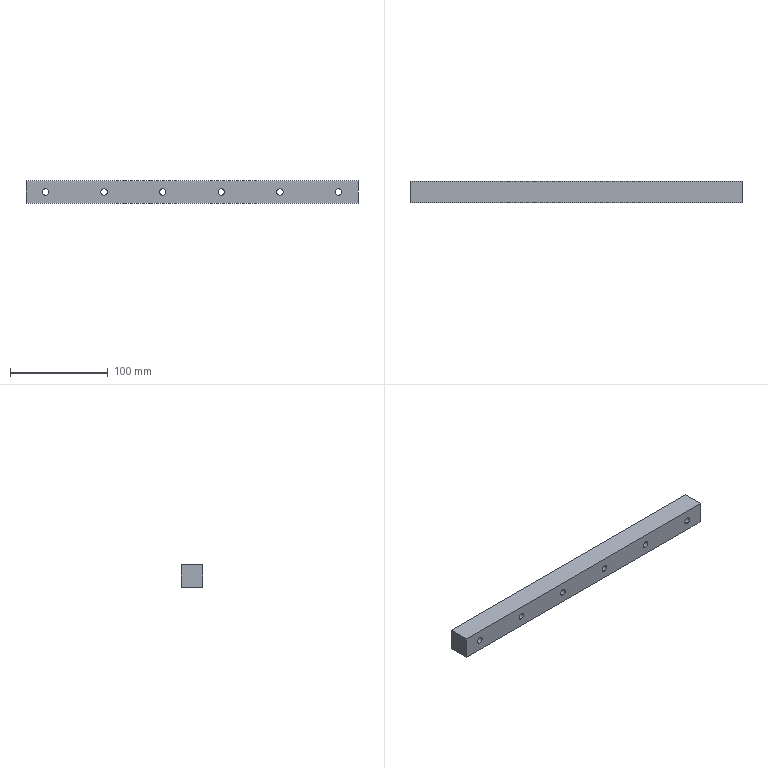Part | SolidWorks | features Extrusion 1, HoleWzd 1, LPattern 1 | 1 solid | 36 faces | box 340 x 22 x 23 mm | volume 165043 mm3 | cylinder 24 | plane 12 | commonest cylinder face diameters 6.6 x12 11 x12
STEP:
#1=CARTESIAN_POINT('',(80.,4.2,-5.5));
#2=VERTEX_POINT('',#1);
#3=CARTESIAN_POINT('',(80.,4.2,5.5));
#4=VERTEX_POINT('',#3);
#5=CARTESIAN_POINT('',(80.,4.2,0.));
#6=DIRECTION('',(0.,1.,0.));
#7=DIRECTION('',(0.,0.,1.));
#8=AXIS2_PLACEMENT_3D('',#5,#6,#7);
#9=CIRCLE('',#8,5.5);
#10=EDGE_CURVE('',#2,#4,#9,.T.);
#11=ORIENTED_EDGE('',*,*,#10,.F.);
#12=CARTESIAN_POINT('',(80.,11.,-5.5));
#13=VERTEX_POINT('',#12);
#14=CARTESIAN_POINT('',(80.,11.,-5.5));
#15=DIRECTION('',(0.,1.,0.));
#16=VECTOR('',#15,1000.);
#17=LINE('',#14,#16);
#18=EDGE_CURVE('',#2,#13,#17,.T.);
#19=ORIENTED_EDGE('',*,*,#18,.T.);
#20=CARTESIAN_POINT('',(80.,11.,5.5));
#21=VERTEX_POINT('',#20);
#22=CARTESIAN_POINT('',(80.,11.,0.));
#23=DIRECTION('',(0.,1.,0.));
#24=DIRECTION('',(0.,0.,1.));
#25=AXIS2_PLACEMENT_3D('',#22,#23,#24);
#26=CIRCLE('',#25,5.5);
#27=EDGE_CURVE('',#13,#21,#26,.T.);
#28=ORIENTED_EDGE('',*,*,#27,.T.);
#29=CARTESIAN_POINT('',(80.,11.,5.5));
#30=DIRECTION('',(0.,1.,0.));
#31=VECTOR('',#30,1000.);
#32=LINE('',#29,#31);
#33=EDGE_CURVE('',#4,#21,#32,.T.);
#34=ORIENTED_EDGE('',*,*,#33,.F.);
#35=EDGE_LOOP('',(#11,#19,#28,#34));
#36=FACE_OUTER_BOUND('',#35,.T.);
#37=CARTESIAN_POINT('',(80.,11.,0.));
#38=DIRECTION('',(0.,1.,0.));
#39=DIRECTION('',(0.,0.,1.));
#40=AXIS2_PLACEMENT_3D('',#37,#38,#39);
#41=CYLINDRICAL_SURFACE('',#40,5.5);
#42=ADVANCED_FACE('',(#36),#41,.F.);
#43=CARTESIAN_POINT('',(80.,-11.,-3.3));
#44=VERTEX_POINT('',#43);
#45=CARTESIAN_POINT('',(80.,-11.,3.3));
#46=VERTEX_POINT('',#45);
#47=CARTESIAN_POINT('',(80.,-11.,0.));
#48=DIRECTION('',(0.,1.,0.));
#49=DIRECTION('',(0.,0.,1.));
#50=AXIS2_PLACEMENT_3D('',#47,#48,#49);
#51=CIRCLE('',#50,3.3);
#52=EDGE_CURVE('',#44,#46,#51,.T.);
#53=ORIENTED_EDGE('',*,*,#52,.F.);
#54=CARTESIAN_POINT('',(80.,4.2,-3.3));
#55=VERTEX_POINT('',#54);
#56=CARTESIAN_POINT('',(80.,11.,-3.3));
#57=DIRECTION('',(0.,1.,0.));
#58=VECTOR('',#57,1000.);
#59=LINE('',#56,#58);
#60=EDGE_CURVE('',#44,#55,#59,.T.);
#61=ORIENTED_EDGE('',*,*,#60,.T.);
#62=CARTESIAN_POINT('',(80.,4.2,3.3));
#63=VERTEX_POINT('',#62);
#64=CARTESIAN_POINT('',(80.,4.2,0.));
#65=DIRECTION('',(0.,1.,0.));
#66=DIRECTION('',(0.,0.,1.));
#67=AXIS2_PLACEMENT_3D('',#64,#65,#66);
#68=CIRCLE('',#67,3.3);
#69=EDGE_CURVE('',#55,#63,#68,.T.);
#70=ORIENTED_EDGE('',*,*,#69,.T.);
#71=CARTESIAN_POINT('',(80.,11.,3.3));
#72=DIRECTION('',(0.,1.,0.));
#73=VECTOR('',#72,1000.);
#74=LINE('',#71,#73);
#75=EDGE_CURVE('',#46,#63,#74,.T.);
#76=ORIENTED_EDGE('',*,*,#75,.F.);
#77=EDGE_LOOP('',(#53,#61,#70,#76));
#78=FACE_OUTER_BOUND('',#77,.T.);
#79=CARTESIAN_POINT('',(80.,11.,0.));
#80=DIRECTION('',(0.,1.,0.));
#81=DIRECTION('',(0.,0.,1.));
#82=AXIS2_PLACEMENT_3D('',#79,#80,#81);
#83=CYLINDRICAL_SURFACE('',#82,3.3);
#84=ADVANCED_FACE('',(#78),#83,.F.);
#85=CARTESIAN_POINT('',(20.,4.2,-5.5));
#86=VERTEX_POINT('',#85);
#87=CARTESIAN_POINT('',(20.,4.2,5.5));
#88=VERTEX_POINT('',#87);
#89=CARTESIAN_POINT('',(20.,4.2,0.));
#90=DIRECTION('',(0.,1.,0.));
#91=DIRECTION('',(0.,0.,1.));
#92=AXIS2_PLACEMENT_3D('',#89,#90,#91);
#93=CIRCLE('',#92,5.5);
#94=EDGE_CURVE('',#86,#88,#93,.T.);
#95=ORIENTED_EDGE('',*,*,#94,.F.);
#96=CARTESIAN_POINT('',(20.,11.,-5.5));
#97=VERTEX_POINT('',#96);
#98=CARTESIAN_POINT('',(20.,11.,-5.5));
#99=DIRECTION('',(0.,1.,0.));
#100=VECTOR('',#99,1000.);
#101=LINE('',#98,#100);
#102=EDGE_CURVE('',#86,#97,#101,.T.);
#103=ORIENTED_EDGE('',*,*,#102,.T.);
#104=CARTESIAN_POINT('',(20.,11.,5.5));
#105=VERTEX_POINT('',#104);
#106=CARTESIAN_POINT('',(20.,11.,0.));
#107=DIRECTION('',(0.,1.,0.));
#108=DIRECTION('',(0.,0.,1.));
#109=AXIS2_PLACEMENT_3D('',#106,#107,#108);
#110=CIRCLE('',#109,5.5);
#111=EDGE_CURVE('',#97,#105,#110,.T.);
#112=ORIENTED_EDGE('',*,*,#111,.T.);
#113=CARTESIAN_POINT('',(20.,11.,5.5));
#114=DIRECTION('',(0.,1.,0.));
#115=VECTOR('',#114,1000.);
#116=LINE('',#113,#115);
#117=EDGE_CURVE('',#88,#105,#116,.T.);
#118=ORIENTED_EDGE('',*,*,#117,.F.);
#119=EDGE_LOOP('',(#95,#103,#112,#118));
#120=FACE_OUTER_BOUND('',#119,.T.);
#121=CARTESIAN_POINT('',(20.,11.,0.));
#122=DIRECTION('',(0.,1.,0.));
#123=DIRECTION('',(0.,0.,1.));
#124=AXIS2_PLACEMENT_3D('',#121,#122,#123);
#125=CYLINDRICAL_SURFACE('',#124,5.5);
#126=ADVANCED_FACE('',(#120),#125,.F.);
#127=CARTESIAN_POINT('',(20.,-11.,-3.3));
#128=VERTEX_POINT('',#127);
#129=CARTESIAN_POINT('',(20.,-11.,3.3));
#130=VERTEX_POINT('',#129);
#131=CARTESIAN_POINT('',(20.,-11.,0.));
#132=DIRECTION('',(0.,1.,0.));
#133=DIRECTION('',(0.,0.,1.));
#134=AXIS2_PLACEMENT_3D('',#131,#132,#133);
#135=CIRCLE('',#134,3.3);
#136=EDGE_CURVE('',#128,#130,#135,.T.);
#137=ORIENTED_EDGE('',*,*,#136,.F.);
#138=CARTESIAN_POINT('',(20.,4.2,-3.3));
#139=VERTEX_POINT('',#138);
#140=CARTESIAN_POINT('',(20.,11.,-3.3));
#141=DIRECTION('',(0.,1.,0.));
#142=VECTOR('',#141,1000.);
#143=LINE('',#140,#142);
#144=EDGE_CURVE('',#128,#139,#143,.T.);
#145=ORIENTED_EDGE('',*,*,#144,.T.);
#146=CARTESIAN_POINT('',(20.,4.2,3.3));
#147=VERTEX_POINT('',#146);
#148=CARTESIAN_POINT('',(20.,4.2,0.));
#149=DIRECTION('',(0.,1.,0.));
#150=DIRECTION('',(0.,0.,1.));
#151=AXIS2_PLACEMENT_3D('',#148,#149,#150);
#152=CIRCLE('',#151,3.3);
#153=EDGE_CURVE('',#139,#147,#152,.T.);
#154=ORIENTED_EDGE('',*,*,#153,.T.);
#155=CARTESIAN_POINT('',(20.,11.,3.3));
#156=DIRECTION('',(0.,1.,0.));
#157=VECTOR('',#156,1000.);
#158=LINE('',#155,#157);
#159=EDGE_CURVE('',#130,#147,#158,.T.);
#160=ORIENTED_EDGE('',*,*,#159,.F.);
#161=EDGE_LOOP('',(#137,#145,#154,#160));
#162=FACE_OUTER_BOUND('',#161,.T.);
#163=CARTESIAN_POINT('',(20.,11.,0.));
#164=DIRECTION('',(0.,1.,0.));
#165=DIRECTION('',(0.,0.,1.));
#166=AXIS2_PLACEMENT_3D('',#163,#164,#165);
#167=CYLINDRICAL_SURFACE('',#166,3.3);
#168=ADVANCED_FACE('',(#162),#167,.F.);
#169=CARTESIAN_POINT('',(140.,-11.,-3.3));
#170=VERTEX_POINT('',#169);
#171=CARTESIAN_POINT('',(140.,-11.,3.3));
#172=VERTEX_POINT('',#171);
#173=CARTESIAN_POINT('',(140.,-11.,0.));
#174=DIRECTION('',(0.,1.,0.));
#175=DIRECTION('',(0.,0.,1.));
#176=AXIS2_PLACEMENT_3D('',#173,#174,#175);
#177=CIRCLE('',#176,3.3);
#178=EDGE_CURVE('',#170,#172,#177,.T.);
#179=ORIENTED_EDGE('',*,*,#178,.F.);
#180=CARTESIAN_POINT('',(140.,4.2,-3.3));
#181=VERTEX_POINT('',#180);
#182=CARTESIAN_POINT('',(140.,11.,-3.3));
#183=DIRECTION('',(0.,1.,0.));
#184=VECTOR('',#183,1000.);
#185=LINE('',#182,#184);
#186=EDGE_CURVE('',#170,#181,#185,.T.);
#187=ORIENTED_EDGE('',*,*,#186,.T.);
#188=CARTESIAN_POINT('',(140.,4.2,3.3));
#189=VERTEX_POINT('',#188);
#190=CARTESIAN_POINT('',(140.,4.2,0.));
#191=DIRECTION('',(0.,1.,0.));
#192=DIRECTION('',(0.,0.,1.));
#193=AXIS2_PLACEMENT_3D('',#190,#191,#192);
#194=CIRCLE('',#193,3.3);
#195=EDGE_CURVE('',#181,#189,#194,.T.);
#196=ORIENTED_EDGE('',*,*,#195,.T.);
#197=CARTESIAN_POINT('',(140.,11.,3.3));
#198=DIRECTION('',(0.,1.,0.));
#199=VECTOR('',#198,1000.);
#200=LINE('',#197,#199);
#201=EDGE_CURVE('',#172,#189,#200,.T.);
#202=ORIENTED_EDGE('',*,*,#201,.F.);
#203=EDGE_LOOP('',(#179,#187,#196,#202));
#204=FACE_OUTER_BOUND('',#203,.T.);
#205=CARTESIAN_POINT('',(140.,11.,0.));
#206=DIRECTION('',(0.,1.,0.));
#207=DIRECTION('',(0.,0.,1.));
#208=AXIS2_PLACEMENT_3D('',#205,#206,#207);
#209=CYLINDRICAL_SURFACE('',#208,3.3);
#210=ADVANCED_FACE('',(#204),#209,.F.);
#211=CARTESIAN_POINT('',(140.,4.2,-5.5));
#212=VERTEX_POINT('',#211);
#213=CARTESIAN_POINT('',(140.,4.2,5.5));
#214=VERTEX_POINT('',#213);
#215=CARTESIAN_POINT('',(140.,4.2,0.));
#216=DIRECTION('',(0.,1.,0.));
#217=DIRECTION('',(0.,0.,1.));
#218=AXIS2_PLACEMENT_3D('',#215,#216,#217);
#219=CIRCLE('',#218,5.5);
#220=EDGE_CURVE('',#212,#214,#219,.T.);
#221=ORIENTED_EDGE('',*,*,#220,.F.);
#222=CARTESIAN_POINT('',(140.,11.,-5.5));
#223=VERTEX_POINT('',#222);
#224=CARTESIAN_POINT('',(140.,11.,-5.5));
#225=DIRECTION('',(0.,1.,0.));
#226=VECTOR('',#225,1000.);
#227=LINE('',#224,#226);
#228=EDGE_CURVE('',#212,#223,#227,.T.);
#229=ORIENTED_EDGE('',*,*,#228,.T.);
#230=CARTESIAN_POINT('',(140.,11.,5.5));
#231=VERTEX_POINT('',#230);
#232=CARTESIAN_POINT('',(140.,11.,0.));
#233=DIRECTION('',(0.,1.,0.));
#234=DIRECTION('',(0.,0.,1.));
#235=AXIS2_PLACEMENT_3D('',#232,#233,#234);
#236=CIRCLE('',#235,5.5);
#237=EDGE_CURVE('',#223,#231,#236,.T.);
#238=ORIENTED_EDGE('',*,*,#237,.T.);
#239=CARTESIAN_POINT('',(140.,11.,5.5));
#240=DIRECTION('',(0.,1.,0.));
#241=VECTOR('',#240,1000.);
#242=LINE('',#239,#241);
#243=EDGE_CURVE('',#214,#231,#242,.T.);
#244=ORIENTED_EDGE('',*,*,#243,.F.);
#245=EDGE_LOOP('',(#221,#229,#238,#244));
#246=FACE_OUTER_BOUND('',#245,.T.);
#247=CARTESIAN_POINT('',(140.,11.,0.));
#248=DIRECTION('',(0.,1.,0.));
#249=DIRECTION('',(0.,0.,1.));
#250=AXIS2_PLACEMENT_3D('',#247,#248,#249);
#251=CYLINDRICAL_SURFACE('',#250,5.5);
#252=ADVANCED_FACE('',(#246),#251,.F.);
#253=CARTESIAN_POINT('',(200.,-11.,-3.3));
#254=VERTEX_POINT('',#253);
#255=CARTESIAN_POINT('',(200.,-11.,3.3));
#256=VERTEX_POINT('',#255);
#257=CARTESIAN_POINT('',(200.,-11.,0.));
#258=DIRECTION('',(0.,1.,0.));
#259=DIRECTION('',(0.,0.,1.));
#260=AXIS2_PLACEMENT_3D('',#257,#258,#259);
#261=CIRCLE('',#260,3.3);
#262=EDGE_CURVE('',#254,#256,#261,.T.);
#263=ORIENTED_EDGE('',*,*,#262,.F.);
#264=CARTESIAN_POINT('',(200.,4.2,-3.3));
#265=VERTEX_POINT('',#264);
#266=CARTESIAN_POINT('',(200.,11.,-3.3));
#267=DIRECTION('',(0.,1.,0.));
#268=VECTOR('',#267,1000.);
#269=LINE('',#266,#268);
#270=EDGE_CURVE('',#254,#265,#269,.T.);
#271=ORIENTED_EDGE('',*,*,#270,.T.);
#272=CARTESIAN_POINT('',(200.,4.2,3.3));
#273=VERTEX_POINT('',#272);
#274=CARTESIAN_POINT('',(200.,4.2,0.));
#275=DIRECTION('',(0.,1.,0.));
#276=DIRECTION('',(0.,0.,1.));
#277=AXIS2_PLACEMENT_3D('',#274,#275,#276);
#278=CIRCLE('',#277,3.3);
#279=EDGE_CURVE('',#265,#273,#278,.T.);
#280=ORIENTED_EDGE('',*,*,#279,.T.);
#281=CARTESIAN_POINT('',(200.,11.,3.3));
#282=DIRECTION('',(0.,1.,0.));
#283=VECTOR('',#282,1000.);
#284=LINE('',#281,#283);
#285=EDGE_CURVE('',#256,#273,#284,.T.);
#286=ORIENTED_EDGE('',*,*,#285,.F.);
#287=EDGE_LOOP('',(#263,#271,#280,#286));
#288=FACE_OUTER_BOUND('',#287,.T.);
#289=CARTESIAN_POINT('',(200.,11.,0.));
#290=DIRECTION('',(0.,1.,0.));
#291=DIRECTION('',(0.,0.,1.));
#292=AXIS2_PLACEMENT_3D('',#289,#290,#291);
#293=CYLINDRICAL_SURFACE('',#292,3.3);
#294=ADVANCED_FACE('',(#288),#293,.F.);
#295=CARTESIAN_POINT('',(200.,4.2,-5.5));
#296=VERTEX_POINT('',#295);
#297=CARTESIAN_POINT('',(200.,4.2,5.5));
#298=VERTEX_POINT('',#297);
#299=CARTESIAN_POINT('',(200.,4.2,0.));
#300=DIRECTION('',(0.,1.,0.));
#301=DIRECTION('',(0.,0.,1.));
#302=AXIS2_PLACEMENT_3D('',#299,#300,#301);
#303=CIRCLE('',#302,5.5);
#304=EDGE_CURVE('',#296,#298,#303,.T.);
#305=ORIENTED_EDGE('',*,*,#304,.F.);
#306=CARTESIAN_POINT('',(200.,11.,-5.5));
#307=VERTEX_POINT('',#306);
#308=CARTESIAN_POINT('',(200.,11.,-5.5));
#309=DIRECTION('',(0.,1.,0.));
#310=VECTOR('',#309,1000.);
#311=LINE('',#308,#310);
#312=EDGE_CURVE('',#296,#307,#311,.T.);
#313=ORIENTED_EDGE('',*,*,#312,.T.);
#314=CARTESIAN_POINT('',(200.,11.,5.5));
#315=VERTEX_POINT('',#314);
#316=CARTESIAN_POINT('',(200.,11.,0.));
#317=DIRECTION('',(0.,1.,0.));
#318=DIRECTION('',(0.,0.,1.));
#319=AXIS2_PLACEMENT_3D('',#316,#317,#318);
#320=CIRCLE('',#319,5.5);
#321=EDGE_CURVE('',#307,#315,#320,.T.);
#322=ORIENTED_EDGE('',*,*,#321,.T.);
#323=CARTESIAN_POINT('',(200.,11.,5.5));
#324=DIRECTION('',(0.,1.,0.));
#325=VECTOR('',#324,1000.);
#326=LINE('',#323,#325);
#327=EDGE_CURVE('',#298,#315,#326,.T.);
#328=ORIENTED_EDGE('',*,*,#327,.F.);
#329=EDGE_LOOP('',(#305,#313,#322,#328));
#330=FACE_OUTER_BOUND('',#329,.T.);
#331=CARTESIAN_POINT('',(200.,11.,0.));
#332=DIRECTION('',(0.,1.,0.));
#333=DIRECTION('',(0.,0.,1.));
#334=AXIS2_PLACEMENT_3D('',#331,#332,#333);
#335=CYLINDRICAL_SURFACE('',#334,5.5);
#336=ADVANCED_FACE('',(#330),#335,.F.);
#337=CARTESIAN_POINT('',(260.,-11.,-3.3));
#338=VERTEX_POINT('',#337);
#339=CARTESIAN_POINT('',(260.,-11.,3.3));
#340=VERTEX_POINT('',#339);
#341=CARTESIAN_POINT('',(260.,-11.,0.));
#342=DIRECTION('',(0.,1.,0.));
#343=DIRECTION('',(0.,0.,1.));
#344=AXIS2_PLACEMENT_3D('',#341,#342,#343);
#345=CIRCLE('',#344,3.3);
#346=EDGE_CURVE('',#338,#340,#345,.T.);
#347=ORIENTED_EDGE('',*,*,#346,.F.);
#348=CARTESIAN_POINT('',(260.,4.2,-3.3));
#349=VERTEX_POINT('',#348);
#350=CARTESIAN_POINT('',(260.,11.,-3.3));
#351=DIRECTION('',(0.,1.,0.));
#352=VECTOR('',#351,1000.);
#353=LINE('',#350,#352);
#354=EDGE_CURVE('',#338,#349,#353,.T.);
#355=ORIENTED_EDGE('',*,*,#354,.T.);
#356=CARTESIAN_POINT('',(260.,4.2,3.3));
#357=VERTEX_POINT('',#356);
#358=CARTESIAN_POINT('',(260.,4.2,0.));
#359=DIRECTION('',(0.,1.,0.));
#360=DIRECTION('',(0.,0.,1.));
#361=AXIS2_PLACEMENT_3D('',#358,#359,#360);
#362=CIRCLE('',#361,3.3);
#363=EDGE_CURVE('',#349,#357,#362,.T.);
#364=ORIENTED_EDGE('',*,*,#363,.T.);
#365=CARTESIAN_POINT('',(260.,11.,3.3));
#366=DIRECTION('',(0.,1.,0.));
#367=VECTOR('',#366,1000.);
#368=LINE('',#365,#367);
#369=EDGE_CURVE('',#340,#357,#368,.T.);
#370=ORIENTED_EDGE('',*,*,#369,.F.);
#371=EDGE_LOOP('',(#347,#355,#364,#370));
#372=FACE_OUTER_BOUND('',#371,.T.);
#373=CARTESIAN_POINT('',(260.,11.,0.));
#374=DIRECTION('',(0.,1.,0.));
#375=DIRECTION('',(0.,0.,1.));
#376=AXIS2_PLACEMENT_3D('',#373,#374,#375);
#377=CYLINDRICAL_SURFACE('',#376,3.3);
#378=ADVANCED_FACE('',(#372),#377,.F.);
#379=CARTESIAN_POINT('',(260.,4.2,-5.5));
#380=VERTEX_POINT('',#379);
#381=CARTESIAN_POINT('',(260.,4.2,5.5));
#382=VERTEX_POINT('',#381);
#383=CARTESIAN_POINT('',(260.,4.2,0.));
#384=DIRECTION('',(0.,1.,0.));
#385=DIRECTION('',(0.,0.,1.));
#386=AXIS2_PLACEMENT_3D('',#383,#384,#385);
#387=CIRCLE('',#386,5.5);
#388=EDGE_CURVE('',#380,#382,#387,.T.);
#389=ORIENTED_EDGE('',*,*,#388,.F.);
#390=CARTESIAN_POINT('',(260.,11.,-5.5));
#391=VERTEX_POINT('',#390);
#392=CARTESIAN_POINT('',(260.,11.,-5.5));
#393=DIRECTION('',(0.,1.,0.));
#394=VECTOR('',#393,1000.);
#395=LINE('',#392,#394);
#396=EDGE_CURVE('',#380,#391,#395,.T.);
#397=ORIENTED_EDGE('',*,*,#396,.T.);
#398=CARTESIAN_POINT('',(260.,11.,5.5));
#399=VERTEX_POINT('',#398);
#400=CARTESIAN_POINT('',(260.,11.,0.));
#401=DIRECTION('',(0.,1.,0.));
#402=DIRECTION('',(0.,0.,1.));
#403=AXIS2_PLACEMENT_3D('',#400,#401,#402);
#404=CIRCLE('',#403,5.5);
#405=EDGE_CURVE('',#391,#399,#404,.T.);
#406=ORIENTED_EDGE('',*,*,#405,.T.);
#407=CARTESIAN_POINT('',(260.,11.,5.5));
#408=DIRECTION('',(0.,1.,0.));
#409=VECTOR('',#408,1000.);
#410=LINE('',#407,#409);
#411=EDGE_CURVE('',#382,#399,#410,.T.);
#412=ORIENTED_EDGE('',*,*,#411,.F.);
#413=EDGE_LOOP('',(#389,#397,#406,#412));
#414=FACE_OUTER_BOUND('',#413,.T.);
#415=CARTESIAN_POINT('',(260.,11.,0.));
#416=DIRECTION('',(0.,1.,0.));
#417=DIRECTION('',(0.,0.,1.));
#418=AXIS2_PLACEMENT_3D('',#415,#416,#417);
#419=CYLINDRICAL_SURFACE('',#418,5.5);
#420=ADVANCED_FACE('',(#414),#419,.F.);
#421=CARTESIAN_POINT('',(320.,-11.,-3.3));
#422=VERTEX_POINT('',#421);
#423=CARTESIAN_POINT('',(320.,-11.,3.3));
#424=VERTEX_POINT('',#423);
#425=CARTESIAN_POINT('',(320.,-11.,0.));
#426=DIRECTION('',(0.,1.,0.));
#427=DIRECTION('',(0.,0.,1.));
#428=AXIS2_PLACEMENT_3D('',#425,#426,#427);
#429=CIRCLE('',#428,3.3);
#430=EDGE_CURVE('',#422,#424,#429,.T.);
#431=ORIENTED_EDGE('',*,*,#430,.F.);
#432=CARTESIAN_POINT('',(320.,4.2,-3.3));
#433=VERTEX_POINT('',#432);
#434=CARTESIAN_POINT('',(320.,11.,-3.3));
#435=DIRECTION('',(0.,1.,0.));
#436=VECTOR('',#435,1000.);
#437=LINE('',#434,#436);
#438=EDGE_CURVE('',#422,#433,#437,.T.);
#439=ORIENTED_EDGE('',*,*,#438,.T.);
#440=CARTESIAN_POINT('',(320.,4.2,3.3));
#441=VERTEX_POINT('',#440);
#442=CARTESIAN_POINT('',(320.,4.2,0.));
#443=DIRECTION('',(0.,1.,0.));
#444=DIRECTION('',(0.,0.,1.));
#445=AXIS2_PLACEMENT_3D('',#442,#443,#444);
#446=CIRCLE('',#445,3.3);
#447=EDGE_CURVE('',#433,#441,#446,.T.);
#448=ORIENTED_EDGE('',*,*,#447,.T.);
#449=CARTESIAN_POINT('',(320.,11.,3.3));
#450=DIRECTION('',(0.,1.,0.));
#451=VECTOR('',#450,1000.);
#452=LINE('',#449,#451);
#453=EDGE_CURVE('',#424,#441,#452,.T.);
#454=ORIENTED_EDGE('',*,*,#453,.F.);
#455=EDGE_LOOP('',(#431,#439,#448,#454));
#456=FACE_OUTER_BOUND('',#455,.T.);
#457=CARTESIAN_POINT('',(320.,11.,0.));
#458=DIRECTION('',(0.,1.,0.));
#459=DIRECTION('',(0.,0.,1.));
#460=AXIS2_PLACEMENT_3D('',#457,#458,#459);
#461=CYLINDRICAL_SURFACE('',#460,3.3);
#462=ADVANCED_FACE('',(#456),#461,.F.);
#463=CARTESIAN_POINT('',(320.,4.2,-5.5));
#464=VERTEX_POINT('',#463);
#465=CARTESIAN_POINT('',(320.,4.2,5.5));
#466=VERTEX_POINT('',#465);
#467=CARTESIAN_POINT('',(320.,4.2,0.));
#468=DIRECTION('',(0.,1.,0.));
#469=DIRECTION('',(0.,0.,1.));
#470=AXIS2_PLACEMENT_3D('',#467,#468,#469);
#471=CIRCLE('',#470,5.5);
#472=EDGE_CURVE('',#464,#466,#471,.T.);
#473=ORIENTED_EDGE('',*,*,#472,.F.);
#474=CARTESIAN_POINT('',(320.,11.,-5.5));
#475=VERTEX_POINT('',#474);
#476=CARTESIAN_POINT('',(320.,11.,-5.5));
#477=DIRECTION('',(0.,1.,0.));
#478=VECTOR('',#477,1000.);
#479=LINE('',#476,#478);
#480=EDGE_CURVE('',#464,#475,#479,.T.);
#481=ORIENTED_EDGE('',*,*,#480,.T.);
#482=CARTESIAN_POINT('',(320.,11.,5.5));
#483=VERTEX_POINT('',#482);
#484=CARTESIAN_POINT('',(320.,11.,0.));
#485=DIRECTION('',(0.,1.,0.));
#486=DIRECTION('',(0.,0.,1.));
#487=AXIS2_PLACEMENT_3D('',#484,#485,#486);
#488=CIRCLE('',#487,5.5);
#489=EDGE_CURVE('',#475,#483,#488,.T.);
#490=ORIENTED_EDGE('',*,*,#489,.T.);
#491=CARTESIAN_POINT('',(320.,11.,5.5));
#492=DIRECTION('',(0.,1.,0.));
#493=VECTOR('',#492,1000.);
#494=LINE('',#491,#493);
#495=EDGE_CURVE('',#466,#483,#494,.T.);
#496=ORIENTED_EDGE('',*,*,#495,.F.);
#497=EDGE_LOOP('',(#473,#481,#490,#496));
#498=FACE_OUTER_BOUND('',#497,.T.);
#499=CARTESIAN_POINT('',(320.,11.,0.));
#500=DIRECTION('',(0.,1.,0.));
#501=DIRECTION('',(0.,0.,1.));
#502=AXIS2_PLACEMENT_3D('',#499,#500,#501);
#503=CYLINDRICAL_SURFACE('',#502,5.5);
#504=ADVANCED_FACE('',(#498),#503,.F.);
#505=ORIENTED_EDGE('',*,*,#480,.F.);
#506=CARTESIAN_POINT('',(320.,4.2,0.));
#507=DIRECTION('',(0.,1.,0.));
#508=DIRECTION('',(0.,0.,1.));
#509=AXIS2_PLACEMENT_3D('',#506,#507,#508);
#510=CIRCLE('',#509,5.5);
#511=EDGE_CURVE('',#466,#464,#510,.T.);
#512=ORIENTED_EDGE('',*,*,#511,.F.);
#513=ORIENTED_EDGE('',*,*,#495,.T.);
#514=CARTESIAN_POINT('',(320.,11.,0.));
#515=DIRECTION('',(0.,1.,0.));
#516=DIRECTION('',(0.,0.,1.));
#517=AXIS2_PLACEMENT_3D('',#514,#515,#516);
#518=CIRCLE('',#517,5.5);
#519=EDGE_CURVE('',#483,#475,#518,.T.);
#520=ORIENTED_EDGE('',*,*,#519,.T.);
#521=EDGE_LOOP('',(#505,#512,#513,#520));
#522=FACE_OUTER_BOUND('',#521,.T.);
#523=CARTESIAN_POINT('',(320.,11.,0.));
#524=DIRECTION('',(0.,1.,0.));
#525=DIRECTION('',(0.,0.,1.));
#526=AXIS2_PLACEMENT_3D('',#523,#524,#525);
#527=CYLINDRICAL_SURFACE('',#526,5.5);
#528=ADVANCED_FACE('',(#522),#527,.F.);
#529=CARTESIAN_POINT('',(320.,4.2,0.));
#530=DIRECTION('',(0.,1.,0.));
#531=DIRECTION('',(0.,0.,1.));
#532=AXIS2_PLACEMENT_3D('',#529,#530,#531);
#533=CIRCLE('',#532,3.3);
#534=EDGE_CURVE('',#441,#433,#533,.T.);
#535=ORIENTED_EDGE('',*,*,#534,.F.);
#536=ORIENTED_EDGE('',*,*,#447,.F.);
#537=EDGE_LOOP('',(#535,#536));
#538=FACE_BOUND('',#537,.T.);
#539=ORIENTED_EDGE('',*,*,#511,.T.);
#540=ORIENTED_EDGE('',*,*,#472,.T.);
#541=EDGE_LOOP('',(#539,#540));
#542=FACE_OUTER_BOUND('',#541,.T.);
#543=CARTESIAN_POINT('',(323.3,4.2,0.));
#544=DIRECTION('',(0.,-1.,0.));
#545=DIRECTION('',(0.,0.,-1.));
#546=AXIS2_PLACEMENT_3D('',#543,#544,#545);
#547=PLANE('',#546);
#548=ADVANCED_FACE('',(#538,#542),#547,.F.);
#549=ORIENTED_EDGE('',*,*,#438,.F.);
#550=CARTESIAN_POINT('',(320.,-11.,0.));
#551=DIRECTION('',(0.,1.,0.));
#552=DIRECTION('',(0.,0.,1.));
#553=AXIS2_PLACEMENT_3D('',#550,#551,#552);
#554=CIRCLE('',#553,3.3);
#555=EDGE_CURVE('',#424,#422,#554,.T.);
#556=ORIENTED_EDGE('',*,*,#555,.F.);
#557=ORIENTED_EDGE('',*,*,#453,.T.);
#558=ORIENTED_EDGE('',*,*,#534,.T.);
#559=EDGE_LOOP('',(#549,#556,#557,#558));
#560=FACE_OUTER_BOUND('',#559,.T.);
#561=CARTESIAN_POINT('',(320.,11.,0.));
#562=DIRECTION('',(0.,1.,0.));
#563=DIRECTION('',(0.,0.,1.));
#564=AXIS2_PLACEMENT_3D('',#561,#562,#563);
#565=CYLINDRICAL_SURFACE('',#564,3.3);
#566=ADVANCED_FACE('',(#560),#565,.F.);
#567=ORIENTED_EDGE('',*,*,#396,.F.);
#568=CARTESIAN_POINT('',(260.,4.2,0.));
#569=DIRECTION('',(0.,1.,0.));
#570=DIRECTION('',(0.,0.,1.));
#571=AXIS2_PLACEMENT_3D('',#568,#569,#570);
#572=CIRCLE('',#571,5.5);
#573=EDGE_CURVE('',#382,#380,#572,.T.);
#574=ORIENTED_EDGE('',*,*,#573,.F.);
#575=ORIENTED_EDGE('',*,*,#411,.T.);
#576=CARTESIAN_POINT('',(260.,11.,0.));
#577=DIRECTION('',(0.,1.,0.));
#578=DIRECTION('',(0.,0.,1.));
#579=AXIS2_PLACEMENT_3D('',#576,#577,#578);
#580=CIRCLE('',#579,5.5);
#581=EDGE_CURVE('',#399,#391,#580,.T.);
#582=ORIENTED_EDGE('',*,*,#581,.T.);
#583=EDGE_LOOP('',(#567,#574,#575,#582));
#584=FACE_OUTER_BOUND('',#583,.T.);
#585=CARTESIAN_POINT('',(260.,11.,0.));
#586=DIRECTION('',(0.,1.,0.));
#587=DIRECTION('',(0.,0.,1.));
#588=AXIS2_PLACEMENT_3D('',#585,#586,#587);
#589=CYLINDRICAL_SURFACE('',#588,5.5);
#590=ADVANCED_FACE('',(#584),#589,.F.);
#591=CARTESIAN_POINT('',(260.,4.2,0.));
#592=DIRECTION('',(0.,1.,0.));
#593=DIRECTION('',(0.,0.,1.));
#594=AXIS2_PLACEMENT_3D('',#591,#592,#593);
#595=CIRCLE('',#594,3.3);
#596=EDGE_CURVE('',#357,#349,#595,.T.);
#597=ORIENTED_EDGE('',*,*,#596,.F.);
#598=ORIENTED_EDGE('',*,*,#363,.F.);
#599=EDGE_LOOP('',(#597,#598));
#600=FACE_BOUND('',#599,.T.);
#601=ORIENTED_EDGE('',*,*,#573,.T.);
#602=ORIENTED_EDGE('',*,*,#388,.T.);
#603=EDGE_LOOP('',(#601,#602));
#604=FACE_OUTER_BOUND('',#603,.T.);
#605=CARTESIAN_POINT('',(263.3,4.2,0.));
#606=DIRECTION('',(0.,-1.,0.));
#607=DIRECTION('',(0.,0.,-1.));
#608=AXIS2_PLACEMENT_3D('',#605,#606,#607);
#609=PLANE('',#608);
#610=ADVANCED_FACE('',(#600,#604),#609,.F.);
#611=ORIENTED_EDGE('',*,*,#354,.F.);
#612=CARTESIAN_POINT('',(260.,-11.,0.));
#613=DIRECTION('',(0.,1.,0.));
#614=DIRECTION('',(0.,0.,1.));
#615=AXIS2_PLACEMENT_3D('',#612,#613,#614);
#616=CIRCLE('',#615,3.3);
#617=EDGE_CURVE('',#340,#338,#616,.T.);
#618=ORIENTED_EDGE('',*,*,#617,.F.);
#619=ORIENTED_EDGE('',*,*,#369,.T.);
#620=ORIENTED_EDGE('',*,*,#596,.T.);
#621=EDGE_LOOP('',(#611,#618,#619,#620));
#622=FACE_OUTER_BOUND('',#621,.T.);
#623=CARTESIAN_POINT('',(260.,11.,0.));
#624=DIRECTION('',(0.,1.,0.));
#625=DIRECTION('',(0.,0.,1.));
#626=AXIS2_PLACEMENT_3D('',#623,#624,#625);
#627=CYLINDRICAL_SURFACE('',#626,3.3);
#628=ADVANCED_FACE('',(#622),#627,.F.);
#629=ORIENTED_EDGE('',*,*,#312,.F.);
#630=CARTESIAN_POINT('',(200.,4.2,0.));
#631=DIRECTION('',(0.,1.,0.));
#632=DIRECTION('',(0.,0.,1.));
#633=AXIS2_PLACEMENT_3D('',#630,#631,#632);
#634=CIRCLE('',#633,5.5);
#635=EDGE_CURVE('',#298,#296,#634,.T.);
#636=ORIENTED_EDGE('',*,*,#635,.F.);
#637=ORIENTED_EDGE('',*,*,#327,.T.);
#638=CARTESIAN_POINT('',(200.,11.,0.));
#639=DIRECTION('',(0.,1.,0.));
#640=DIRECTION('',(0.,0.,1.));
#641=AXIS2_PLACEMENT_3D('',#638,#639,#640);
#642=CIRCLE('',#641,5.5);
#643=EDGE_CURVE('',#315,#307,#642,.T.);
#644=ORIENTED_EDGE('',*,*,#643,.T.);
#645=EDGE_LOOP('',(#629,#636,#637,#644));
#646=FACE_OUTER_BOUND('',#645,.T.);
#647=CARTESIAN_POINT('',(200.,11.,0.));
#648=DIRECTION('',(0.,1.,0.));
#649=DIRECTION('',(0.,0.,1.));
#650=AXIS2_PLACEMENT_3D('',#647,#648,#649);
#651=CYLINDRICAL_SURFACE('',#650,5.5);
#652=ADVANCED_FACE('',(#646),#651,.F.);
#653=CARTESIAN_POINT('',(200.,4.2,0.));
#654=DIRECTION('',(0.,1.,0.));
#655=DIRECTION('',(0.,0.,1.));
#656=AXIS2_PLACEMENT_3D('',#653,#654,#655);
#657=CIRCLE('',#656,3.3);
#658=EDGE_CURVE('',#273,#265,#657,.T.);
#659=ORIENTED_EDGE('',*,*,#658,.F.);
#660=ORIENTED_EDGE('',*,*,#279,.F.);
#661=EDGE_LOOP('',(#659,#660));
#662=FACE_BOUND('',#661,.T.);
#663=ORIENTED_EDGE('',*,*,#635,.T.);
#664=ORIENTED_EDGE('',*,*,#304,.T.);
#665=EDGE_LOOP('',(#663,#664));
#666=FACE_OUTER_BOUND('',#665,.T.);
#667=CARTESIAN_POINT('',(203.3,4.2,0.));
#668=DIRECTION('',(0.,-1.,0.));
#669=DIRECTION('',(0.,0.,-1.));
#670=AXIS2_PLACEMENT_3D('',#667,#668,#669);
#671=PLANE('',#670);
#672=ADVANCED_FACE('',(#662,#666),#671,.F.);
#673=ORIENTED_EDGE('',*,*,#270,.F.);
#674=CARTESIAN_POINT('',(200.,-11.,0.));
#675=DIRECTION('',(0.,1.,0.));
#676=DIRECTION('',(0.,0.,1.));
#677=AXIS2_PLACEMENT_3D('',#674,#675,#676);
#678=CIRCLE('',#677,3.3);
#679=EDGE_CURVE('',#256,#254,#678,.T.);
#680=ORIENTED_EDGE('',*,*,#679,.F.);
#681=ORIENTED_EDGE('',*,*,#285,.T.);
#682=ORIENTED_EDGE('',*,*,#658,.T.);
#683=EDGE_LOOP('',(#673,#680,#681,#682));
#684=FACE_OUTER_BOUND('',#683,.T.);
#685=CARTESIAN_POINT('',(200.,11.,0.));
#686=DIRECTION('',(0.,1.,0.));
#687=DIRECTION('',(0.,0.,1.));
#688=AXIS2_PLACEMENT_3D('',#685,#686,#687);
#689=CYLINDRICAL_SURFACE('',#688,3.3);
#690=ADVANCED_FACE('',(#684),#689,.F.);
#691=ORIENTED_EDGE('',*,*,#228,.F.);
#692=CARTESIAN_POINT('',(140.,4.2,0.));
#693=DIRECTION('',(0.,1.,0.));
#694=DIRECTION('',(0.,0.,1.));
#695=AXIS2_PLACEMENT_3D('',#692,#693,#694);
#696=CIRCLE('',#695,5.5);
#697=EDGE_CURVE('',#214,#212,#696,.T.);
#698=ORIENTED_EDGE('',*,*,#697,.F.);
#699=ORIENTED_EDGE('',*,*,#243,.T.);
#700=CARTESIAN_POINT('',(140.,11.,0.));
#701=DIRECTION('',(0.,1.,0.));
#702=DIRECTION('',(0.,0.,1.));
#703=AXIS2_PLACEMENT_3D('',#700,#701,#702);
#704=CIRCLE('',#703,5.5);
#705=EDGE_CURVE('',#231,#223,#704,.T.);
#706=ORIENTED_EDGE('',*,*,#705,.T.);
#707=EDGE_LOOP('',(#691,#698,#699,#706));
#708=FACE_OUTER_BOUND('',#707,.T.);
#709=CARTESIAN_POINT('',(140.,11.,0.));
#710=DIRECTION('',(0.,1.,0.));
#711=DIRECTION('',(0.,0.,1.));
#712=AXIS2_PLACEMENT_3D('',#709,#710,#711);
#713=CYLINDRICAL_SURFACE('',#712,5.5);
#714=ADVANCED_FACE('',(#708),#713,.F.);
#715=CARTESIAN_POINT('',(140.,4.2,0.));
#716=DIRECTION('',(0.,1.,0.));
#717=DIRECTION('',(0.,0.,1.));
#718=AXIS2_PLACEMENT_3D('',#715,#716,#717);
#719=CIRCLE('',#718,3.3);
#720=EDGE_CURVE('',#189,#181,#719,.T.);
#721=ORIENTED_EDGE('',*,*,#720,.F.);
#722=ORIENTED_EDGE('',*,*,#195,.F.);
#723=EDGE_LOOP('',(#721,#722));
#724=FACE_BOUND('',#723,.T.);
#725=ORIENTED_EDGE('',*,*,#697,.T.);
#726=ORIENTED_EDGE('',*,*,#220,.T.);
#727=EDGE_LOOP('',(#725,#726));
#728=FACE_OUTER_BOUND('',#727,.T.);
#729=CARTESIAN_POINT('',(143.3,4.2,0.));
#730=DIRECTION('',(0.,-1.,0.));
#731=DIRECTION('',(0.,0.,-1.));
#732=AXIS2_PLACEMENT_3D('',#729,#730,#731);
#733=PLANE('',#732);
#734=ADVANCED_FACE('',(#724,#728),#733,.F.);
#735=ORIENTED_EDGE('',*,*,#186,.F.);
#736=CARTESIAN_POINT('',(140.,-11.,0.));
#737=DIRECTION('',(0.,1.,0.));
#738=DIRECTION('',(0.,0.,1.));
#739=AXIS2_PLACEMENT_3D('',#736,#737,#738);
#740=CIRCLE('',#739,3.3);
#741=EDGE_CURVE('',#172,#170,#740,.T.);
#742=ORIENTED_EDGE('',*,*,#741,.F.);
#743=ORIENTED_EDGE('',*,*,#201,.T.);
#744=ORIENTED_EDGE('',*,*,#720,.T.);
#745=EDGE_LOOP('',(#735,#742,#743,#744));
#746=FACE_OUTER_BOUND('',#745,.T.);
#747=CARTESIAN_POINT('',(140.,11.,0.));
#748=DIRECTION('',(0.,1.,0.));
#749=DIRECTION('',(0.,0.,1.));
#750=AXIS2_PLACEMENT_3D('',#747,#748,#749);
#751=CYLINDRICAL_SURFACE('',#750,3.3);
#752=ADVANCED_FACE('',(#746),#751,.F.);
#753=CARTESIAN_POINT('',(0.,-11.,-11.5));
#754=VERTEX_POINT('',#753);
#755=CARTESIAN_POINT('',(0.,11.,-11.5));
#756=VERTEX_POINT('',#755);
#757=CARTESIAN_POINT('',(0.,11.,-11.5));
#758=DIRECTION('',(0.,1.,0.));
#759=VECTOR('',#758,1000.);
#760=LINE('',#757,#759);
#761=EDGE_CURVE('',#754,#756,#760,.T.);
#762=ORIENTED_EDGE('',*,*,#761,.T.);
#763=CARTESIAN_POINT('',(340.,11.,-11.5));
#764=VERTEX_POINT('',#763);
#765=CARTESIAN_POINT('',(340.,11.,-11.5));
#766=DIRECTION('',(-1.,0.,0.));
#767=VECTOR('',#766,1000.);
#768=LINE('',#765,#767);
#769=EDGE_CURVE('',#764,#756,#768,.T.);
#770=ORIENTED_EDGE('',*,*,#769,.F.);
#771=CARTESIAN_POINT('',(340.,-11.,-11.5));
#772=VERTEX_POINT('',#771);
#773=CARTESIAN_POINT('',(340.,11.,-11.5));
#774=DIRECTION('',(0.,1.,0.));
#775=VECTOR('',#774,1000.);
#776=LINE('',#773,#775);
#777=EDGE_CURVE('',#772,#764,#776,.T.);
#778=ORIENTED_EDGE('',*,*,#777,.F.);
#779=CARTESIAN_POINT('',(340.,-11.,-11.5));
#780=DIRECTION('',(-1.,0.,0.));
#781=VECTOR('',#780,1000.);
#782=LINE('',#779,#781);
#783=EDGE_CURVE('',#772,#754,#782,.T.);
#784=ORIENTED_EDGE('',*,*,#783,.T.);
#785=EDGE_LOOP('',(#762,#770,#778,#784));
#786=FACE_OUTER_BOUND('',#785,.T.);
#787=CARTESIAN_POINT('',(340.,11.,-11.5));
#788=DIRECTION('',(0.,0.,1.));
#789=DIRECTION('',(0.,-1.,0.));
#790=AXIS2_PLACEMENT_3D('',#787,#788,#789);
#791=PLANE('',#790);
#792=ADVANCED_FACE('',(#786),#791,.F.);
#793=CARTESIAN_POINT('',(80.,11.,0.));
#794=DIRECTION('',(0.,1.,0.));
#795=DIRECTION('',(0.,0.,1.));
#796=AXIS2_PLACEMENT_3D('',#793,#794,#795);
#797=CIRCLE('',#796,5.5);
#798=EDGE_CURVE('',#21,#13,#797,.T.);
#799=ORIENTED_EDGE('',*,*,#798,.F.);
#800=ORIENTED_EDGE('',*,*,#27,.F.);
#801=EDGE_LOOP('',(#799,#800));
#802=FACE_BOUND('',#801,.T.);
#803=CARTESIAN_POINT('',(20.,11.,0.));
#804=DIRECTION('',(0.,1.,0.));
#805=DIRECTION('',(0.,0.,1.));
#806=AXIS2_PLACEMENT_3D('',#803,#804,#805);
#807=CIRCLE('',#806,5.5);
#808=EDGE_CURVE('',#105,#97,#807,.T.);
#809=ORIENTED_EDGE('',*,*,#808,.F.);
#810=ORIENTED_EDGE('',*,*,#111,.F.);
#811=EDGE_LOOP('',(#809,#810));
#812=FACE_BOUND('',#811,.T.);
#813=CARTESIAN_POINT('',(0.,11.,11.5));
#814=VERTEX_POINT('',#813);
#815=CARTESIAN_POINT('',(0.,11.,11.5));
#816=DIRECTION('',(0.,0.,1.));
#817=VECTOR('',#816,1000.);
#818=LINE('',#815,#817);
#819=EDGE_CURVE('',#756,#814,#818,.T.);
#820=ORIENTED_EDGE('',*,*,#819,.T.);
#821=CARTESIAN_POINT('',(340.,11.,11.5));
#822=VERTEX_POINT('',#821);
#823=CARTESIAN_POINT('',(340.,11.,11.5));
#824=DIRECTION('',(-1.,0.,0.));
#825=VECTOR('',#824,1000.);
#826=LINE('',#823,#825);
#827=EDGE_CURVE('',#822,#814,#826,.T.);
#828=ORIENTED_EDGE('',*,*,#827,.F.);
#829=CARTESIAN_POINT('',(340.,11.,11.5));
#830=DIRECTION('',(0.,0.,1.));
#831=VECTOR('',#830,1000.);
#832=LINE('',#829,#831);
#833=EDGE_CURVE('',#764,#822,#832,.T.);
#834=ORIENTED_EDGE('',*,*,#833,.F.);
#835=ORIENTED_EDGE('',*,*,#769,.T.);
#836=EDGE_LOOP('',(#820,#828,#834,#835));
#837=FACE_OUTER_BOUND('',#836,.T.);
#838=ORIENTED_EDGE('',*,*,#705,.F.);
#839=ORIENTED_EDGE('',*,*,#237,.F.);
#840=EDGE_LOOP('',(#838,#839));
#841=FACE_BOUND('',#840,.T.);
#842=ORIENTED_EDGE('',*,*,#643,.F.);
#843=ORIENTED_EDGE('',*,*,#321,.F.);
#844=EDGE_LOOP('',(#842,#843));
#845=FACE_BOUND('',#844,.T.);
#846=ORIENTED_EDGE('',*,*,#581,.F.);
#847=ORIENTED_EDGE('',*,*,#405,.F.);
#848=EDGE_LOOP('',(#846,#847));
#849=FACE_BOUND('',#848,.T.);
#850=ORIENTED_EDGE('',*,*,#519,.F.);
#851=ORIENTED_EDGE('',*,*,#489,.F.);
#852=EDGE_LOOP('',(#850,#851));
#853=FACE_BOUND('',#852,.T.);
#854=CARTESIAN_POINT('',(340.,11.,11.5));
#855=DIRECTION('',(0.,-1.,0.));
#856=DIRECTION('',(0.,0.,-1.));
#857=AXIS2_PLACEMENT_3D('',#854,#855,#856);
#858=PLANE('',#857);
#859=ADVANCED_FACE('',(#802,#812,#837,#841,#845,#849,#853),#858,.F.);
#860=CARTESIAN_POINT('',(0.,-11.,11.5));
#861=VERTEX_POINT('',#860);
#862=CARTESIAN_POINT('',(0.,11.,11.5));
#863=DIRECTION('',(0.,-1.,0.));
#864=VECTOR('',#863,1000.);
#865=LINE('',#862,#864);
#866=EDGE_CURVE('',#814,#861,#865,.T.);
#867=ORIENTED_EDGE('',*,*,#866,.T.);
#868=CARTESIAN_POINT('',(340.,-11.,11.5));
#869=VERTEX_POINT('',#868);
#870=CARTESIAN_POINT('',(340.,-11.,11.5));
#871=DIRECTION('',(-1.,0.,0.));
#872=VECTOR('',#871,1000.);
#873=LINE('',#870,#872);
#874=EDGE_CURVE('',#869,#861,#873,.T.);
#875=ORIENTED_EDGE('',*,*,#874,.F.);
#876=CARTESIAN_POINT('',(340.,11.,11.5));
#877=DIRECTION('',(0.,-1.,0.));
#878=VECTOR('',#877,1000.);
#879=LINE('',#876,#878);
#880=EDGE_CURVE('',#822,#869,#879,.T.);
#881=ORIENTED_EDGE('',*,*,#880,.F.);
#882=ORIENTED_EDGE('',*,*,#827,.T.);
#883=EDGE_LOOP('',(#867,#875,#881,#882));
#884=FACE_OUTER_BOUND('',#883,.T.);
#885=CARTESIAN_POINT('',(340.,11.,11.5));
#886=DIRECTION('',(0.,0.,-1.));
#887=DIRECTION('',(0.,1.,0.));
#888=AXIS2_PLACEMENT_3D('',#885,#886,#887);
#889=PLANE('',#888);
#890=ADVANCED_FACE('',(#884),#889,.F.);
#891=CARTESIAN_POINT('',(80.,-11.,0.));
#892=DIRECTION('',(0.,1.,0.));
#893=DIRECTION('',(0.,0.,1.));
#894=AXIS2_PLACEMENT_3D('',#891,#892,#893);
#895=CIRCLE('',#894,3.3);
#896=EDGE_CURVE('',#46,#44,#895,.T.);
#897=ORIENTED_EDGE('',*,*,#896,.T.);
#898=ORIENTED_EDGE('',*,*,#52,.T.);
#899=EDGE_LOOP('',(#897,#898));
#900=FACE_BOUND('',#899,.T.);
#901=CARTESIAN_POINT('',(20.,-11.,0.));
#902=DIRECTION('',(0.,1.,0.));
#903=DIRECTION('',(0.,0.,1.));
#904=AXIS2_PLACEMENT_3D('',#901,#902,#903);
#905=CIRCLE('',#904,3.3);
#906=EDGE_CURVE('',#130,#128,#905,.T.);
#907=ORIENTED_EDGE('',*,*,#906,.T.);
#908=ORIENTED_EDGE('',*,*,#136,.T.);
#909=EDGE_LOOP('',(#907,#908));
#910=FACE_BOUND('',#909,.T.);
#911=CARTESIAN_POINT('',(0.,-11.,11.5));
#912=DIRECTION('',(0.,0.,-1.));
#913=VECTOR('',#912,1000.);
#914=LINE('',#911,#913);
#915=EDGE_CURVE('',#861,#754,#914,.T.);
#916=ORIENTED_EDGE('',*,*,#915,.T.);
#917=ORIENTED_EDGE('',*,*,#783,.F.);
#918=CARTESIAN_POINT('',(340.,-11.,11.5));
#919=DIRECTION('',(0.,0.,-1.));
#920=VECTOR('',#919,1000.);
#921=LINE('',#918,#920);
#922=EDGE_CURVE('',#869,#772,#921,.T.);
#923=ORIENTED_EDGE('',*,*,#922,.F.);
#924=ORIENTED_EDGE('',*,*,#874,.T.);
#925=EDGE_LOOP('',(#916,#917,#923,#924));
#926=FACE_OUTER_BOUND('',#925,.T.);
#927=ORIENTED_EDGE('',*,*,#741,.T.);
#928=ORIENTED_EDGE('',*,*,#178,.T.);
#929=EDGE_LOOP('',(#927,#928));
#930=FACE_BOUND('',#929,.T.);
#931=ORIENTED_EDGE('',*,*,#679,.T.);
#932=ORIENTED_EDGE('',*,*,#262,.T.);
#933=EDGE_LOOP('',(#931,#932));
#934=FACE_BOUND('',#933,.T.);
#935=ORIENTED_EDGE('',*,*,#617,.T.);
#936=ORIENTED_EDGE('',*,*,#346,.T.);
#937=EDGE_LOOP('',(#935,#936));
#938=FACE_BOUND('',#937,.T.);
#939=ORIENTED_EDGE('',*,*,#555,.T.);
#940=ORIENTED_EDGE('',*,*,#430,.T.);
#941=EDGE_LOOP('',(#939,#940));
#942=FACE_BOUND('',#941,.T.);
#943=CARTESIAN_POINT('',(340.,-11.,11.5));
#944=DIRECTION('',(0.,1.,0.));
#945=DIRECTION('',(0.,0.,1.));
#946=AXIS2_PLACEMENT_3D('',#943,#944,#945);
#947=PLANE('',#946);
#948=ADVANCED_FACE('',(#900,#910,#926,#930,#934,#938,#942),#947,.F.);
#949=ORIENTED_EDGE('',*,*,#777,.T.);
#950=ORIENTED_EDGE('',*,*,#833,.T.);
#951=ORIENTED_EDGE('',*,*,#880,.T.);
#952=ORIENTED_EDGE('',*,*,#922,.T.);
#953=EDGE_LOOP('',(#949,#950,#951,#952));
#954=FACE_OUTER_BOUND('',#953,.T.);
#955=CARTESIAN_POINT('',(340.,0.,0.));
#956=DIRECTION('',(1.,0.,0.));
#957=DIRECTION('',(0.,0.,-1.));
#958=AXIS2_PLACEMENT_3D('',#955,#956,#957);
#959=PLANE('',#958);
#960=ADVANCED_FACE('',(#954),#959,.T.);
#961=ORIENTED_EDGE('',*,*,#761,.F.);
#962=ORIENTED_EDGE('',*,*,#915,.F.);
#963=ORIENTED_EDGE('',*,*,#866,.F.);
#964=ORIENTED_EDGE('',*,*,#819,.F.);
#965=EDGE_LOOP('',(#961,#962,#963,#964));
#966=FACE_OUTER_BOUND('',#965,.T.);
#967=CARTESIAN_POINT('',(0.,0.,0.));
#968=DIRECTION('',(1.,0.,0.));
#969=DIRECTION('',(0.,0.,-1.));
#970=AXIS2_PLACEMENT_3D('',#967,#968,#969);
#971=PLANE('',#970);
#972=ADVANCED_FACE('',(#966),#971,.F.);
#973=ORIENTED_EDGE('',*,*,#144,.F.);
#974=ORIENTED_EDGE('',*,*,#906,.F.);
#975=ORIENTED_EDGE('',*,*,#159,.T.);
#976=CARTESIAN_POINT('',(20.,4.2,0.));
#977=DIRECTION('',(0.,1.,0.));
#978=DIRECTION('',(0.,0.,1.));
#979=AXIS2_PLACEMENT_3D('',#976,#977,#978);
#980=CIRCLE('',#979,3.3);
#981=EDGE_CURVE('',#147,#139,#980,.T.);
#982=ORIENTED_EDGE('',*,*,#981,.T.);
#983=EDGE_LOOP('',(#973,#974,#975,#982));
#984=FACE_OUTER_BOUND('',#983,.T.);
#985=CARTESIAN_POINT('',(20.,11.,0.));
#986=DIRECTION('',(0.,1.,0.));
#987=DIRECTION('',(0.,0.,1.));
#988=AXIS2_PLACEMENT_3D('',#985,#986,#987);
#989=CYLINDRICAL_SURFACE('',#988,3.3);
#990=ADVANCED_FACE('',(#984),#989,.F.);
#991=ORIENTED_EDGE('',*,*,#981,.F.);
#992=ORIENTED_EDGE('',*,*,#153,.F.);
#993=EDGE_LOOP('',(#991,#992));
#994=FACE_BOUND('',#993,.T.);
#995=CARTESIAN_POINT('',(20.,4.2,0.));
#996=DIRECTION('',(0.,1.,0.));
#997=DIRECTION('',(0.,0.,1.));
#998=AXIS2_PLACEMENT_3D('',#995,#996,#997);
#999=CIRCLE('',#998,5.5);
#1000=EDGE_CURVE('',#88,#86,#999,.T.);
#1001=ORIENTED_EDGE('',*,*,#1000,.T.);
#1002=ORIENTED_EDGE('',*,*,#94,.T.);
#1003=EDGE_LOOP('',(#1001,#1002));
#1004=FACE_OUTER_BOUND('',#1003,.T.);
#1005=CARTESIAN_POINT('',(23.3,4.2,0.));
#1006=DIRECTION('',(0.,-1.,0.));
#1007=DIRECTION('',(0.,0.,-1.));
#1008=AXIS2_PLACEMENT_3D('',#1005,#1006,#1007);
#1009=PLANE('',#1008);
#1010=ADVANCED_FACE('',(#994,#1004),#1009,.F.);
#1011=ORIENTED_EDGE('',*,*,#102,.F.);
#1012=ORIENTED_EDGE('',*,*,#1000,.F.);
#1013=ORIENTED_EDGE('',*,*,#117,.T.);
#1014=ORIENTED_EDGE('',*,*,#808,.T.);
#1015=EDGE_LOOP('',(#1011,#1012,#1013,#1014));
#1016=FACE_OUTER_BOUND('',#1015,.T.);
#1017=CARTESIAN_POINT('',(20.,11.,0.));
#1018=DIRECTION('',(0.,1.,0.));
#1019=DIRECTION('',(0.,0.,1.));
#1020=AXIS2_PLACEMENT_3D('',#1017,#1018,#1019);
#1021=CYLINDRICAL_SURFACE('',#1020,5.5);
#1022=ADVANCED_FACE('',(#1016),#1021,.F.);
#1023=ORIENTED_EDGE('',*,*,#60,.F.);
#1024=ORIENTED_EDGE('',*,*,#896,.F.);
#1025=ORIENTED_EDGE('',*,*,#75,.T.);
#1026=CARTESIAN_POINT('',(80.,4.2,0.));
#1027=DIRECTION('',(0.,1.,0.));
#1028=DIRECTION('',(0.,0.,1.));
#1029=AXIS2_PLACEMENT_3D('',#1026,#1027,#1028);
#1030=CIRCLE('',#1029,3.3);
#1031=EDGE_CURVE('',#63,#55,#1030,.T.);
#1032=ORIENTED_EDGE('',*,*,#1031,.T.);
#1033=EDGE_LOOP('',(#1023,#1024,#1025,#1032));
#1034=FACE_OUTER_BOUND('',#1033,.T.);
#1035=CARTESIAN_POINT('',(80.,11.,0.));
#1036=DIRECTION('',(0.,1.,0.));
#1037=DIRECTION('',(0.,0.,1.));
#1038=AXIS2_PLACEMENT_3D('',#1035,#1036,#1037);
#1039=CYLINDRICAL_SURFACE('',#1038,3.3);
#1040=ADVANCED_FACE('',(#1034),#1039,.F.);
#1041=ORIENTED_EDGE('',*,*,#1031,.F.);
#1042=ORIENTED_EDGE('',*,*,#69,.F.);
#1043=EDGE_LOOP('',(#1041,#1042));
#1044=FACE_BOUND('',#1043,.T.);
#1045=CARTESIAN_POINT('',(80.,4.2,0.));
#1046=DIRECTION('',(0.,1.,0.));
#1047=DIRECTION('',(0.,0.,1.));
#1048=AXIS2_PLACEMENT_3D('',#1045,#1046,#1047);
#1049=CIRCLE('',#1048,5.5);
#1050=EDGE_CURVE('',#4,#2,#1049,.T.);
#1051=ORIENTED_EDGE('',*,*,#1050,.T.);
#1052=ORIENTED_EDGE('',*,*,#10,.T.);
#1053=EDGE_LOOP('',(#1051,#1052));
#1054=FACE_OUTER_BOUND('',#1053,.T.);
#1055=CARTESIAN_POINT('',(83.3,4.2,0.));
#1056=DIRECTION('',(0.,-1.,0.));
#1057=DIRECTION('',(0.,0.,-1.));
#1058=AXIS2_PLACEMENT_3D('',#1055,#1056,#1057);
#1059=PLANE('',#1058);
#1060=ADVANCED_FACE('',(#1044,#1054),#1059,.F.);
#1061=ORIENTED_EDGE('',*,*,#18,.F.);
#1062=ORIENTED_EDGE('',*,*,#1050,.F.);
#1063=ORIENTED_EDGE('',*,*,#33,.T.);
#1064=ORIENTED_EDGE('',*,*,#798,.T.);
#1065=EDGE_LOOP('',(#1061,#1062,#1063,#1064));
#1066=FACE_OUTER_BOUND('',#1065,.T.);
#1067=CARTESIAN_POINT('',(80.,11.,0.));
#1068=DIRECTION('',(0.,1.,0.));
#1069=DIRECTION('',(0.,0.,1.));
#1070=AXIS2_PLACEMENT_3D('',#1067,#1068,#1069);
#1071=CYLINDRICAL_SURFACE('',#1070,5.5);
#1072=ADVANCED_FACE('',(#1066),#1071,.F.);
#1073=CLOSED_SHELL('',(#42,#84,#126,#168,#210,#252,#294,#336,#378,#420,#462,#504,#528,#548,#566,#590,#610,#628,#652,#672,#690,#714,#734,#752,#792,#859,#890,#948,#960,#972,#990,#1010,#1022,#1040,#1060,#1072));
#1074=MANIFOLD_SOLID_BREP('',#1073);
#1075=CARTESIAN_POINT('',(0.,0.,0.));
#1076=DIRECTION('',(0.,0.,1.));
#1077=DIRECTION('',(1.,0.,0.));
#1078=AXIS2_PLACEMENT_3D('',#1075,#1076,#1077);
#1079=(LENGTH_UNIT()NAMED_UNIT(*)SI_UNIT(.MILLI.,.METRE.));
#1080=UNCERTAINTY_MEASURE_WITH_UNIT(LENGTH_MEASURE(0.00001),#1079,'','');
#1081=(NAMED_UNIT(*)PLANE_ANGLE_UNIT()SI_UNIT($,.RADIAN.));
#1082=(NAMED_UNIT(*)SI_UNIT($,.STERADIAN.)SOLID_ANGLE_UNIT());
#1083=(GEOMETRIC_REPRESENTATION_CONTEXT(3)GLOBAL_UNCERTAINTY_ASSIGNED_CONTEXT((#1080))GLOBAL_UNIT_ASSIGNED_CONTEXT((#1079,#1081,#1082))REPRESENTATION_CONTEXT('',''));
#1084=ADVANCED_BREP_SHAPE_REPRESENTATION('',(#1074,#1078),#1083);